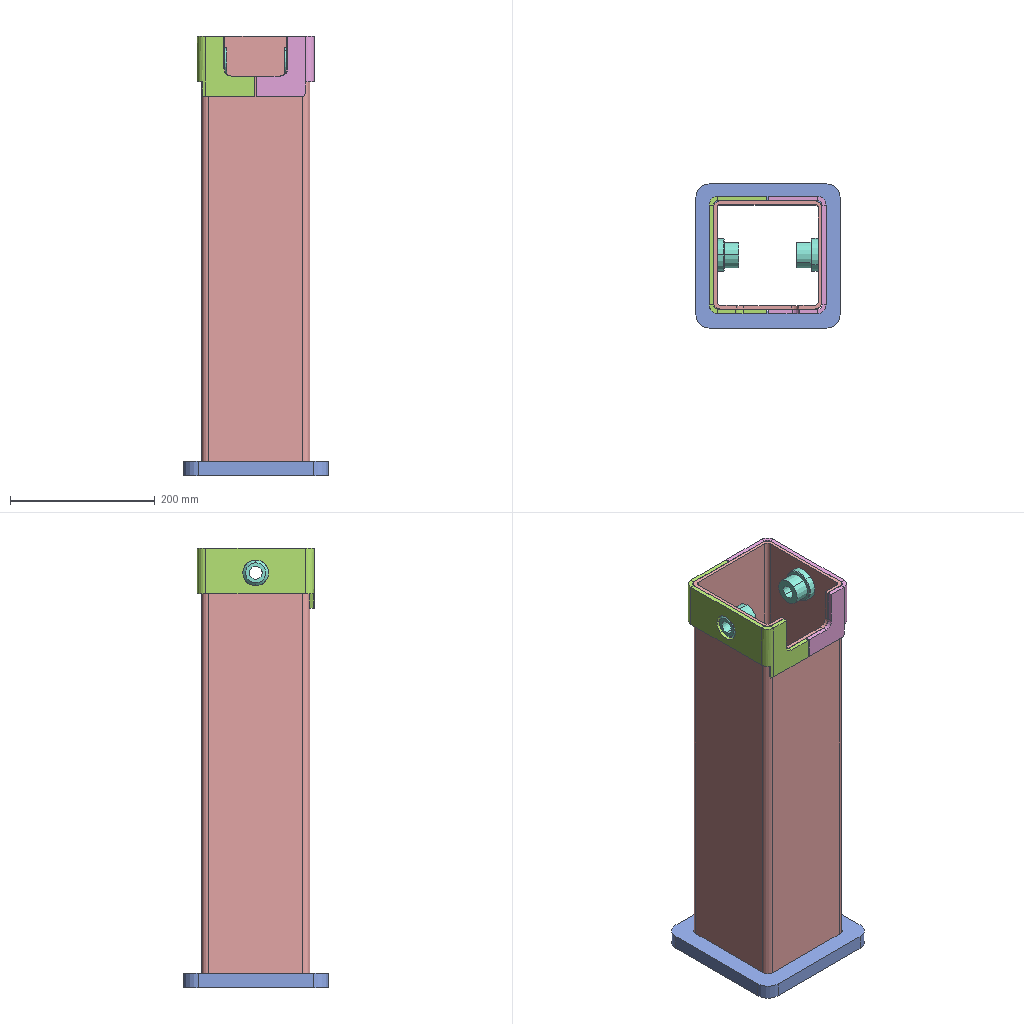Assembly | SolidWorks | 5 different items | 6 placed | box 200 x 200 x 608 mm
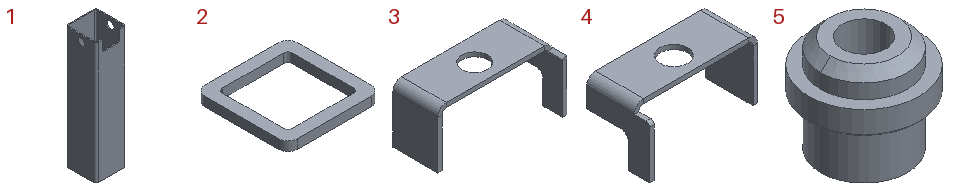Parts list (item | quantity | size | volume | features):
1 | x1 | 150 x 150 x 608 mm | 1690442 mm3 | features Fillet 3, ICE 2, Extrusion 1
2 | x1 | 200 x 200 x 20 mm | 338830 mm3 | features Fillet 2, Extrusion 1
3 | x1 | 162 x 83 x 80 mm | 102695 mm3 | features ICE 3, Fillet 1, FlatPattern 1, SMBaseFlange 1, SheetMetal 1
4 | x1 | 162 x 83 x 80 mm | 102219 mm3 | features ICE 3, Fillet 2, FlatPattern 1, SMBaseFlange 1, SheetMetal 1
5 | x2 | 46 x 46 x 40 mm | 36068 mm3 | features ICE 3, Chamfer 2, Extrusion 1
Mates (type | each side: item.copy, entity, surface, feature):
Coincident | 1.1 face plane Boss-Extrude1 | 2.1 face plane Boss-Extrude1 | 3 times
Coincident | 1.1 face plane Boss-Extrude1 | 3.1 face plane Base-Flange1 | 3 times
Coincident | 3.1 face plane Base-Flange1 | 4.1 face plane Base-Flange1 | 2 times
Coincident | 1.1 face plane Boss-Extrude1 | 4.1 face plane Base-Flange1
Coincident | 1.1 face plane Boss-Extrude1 | 5.1 face plane Boss-Extrude2
Concentric | 1.1 edge | 5.1 edge
Coincident | 1.1 face plane Boss-Extrude1 | 5.2 face plane Boss-Extrude2
Concentric | 1.1 edge | 5.2 edge